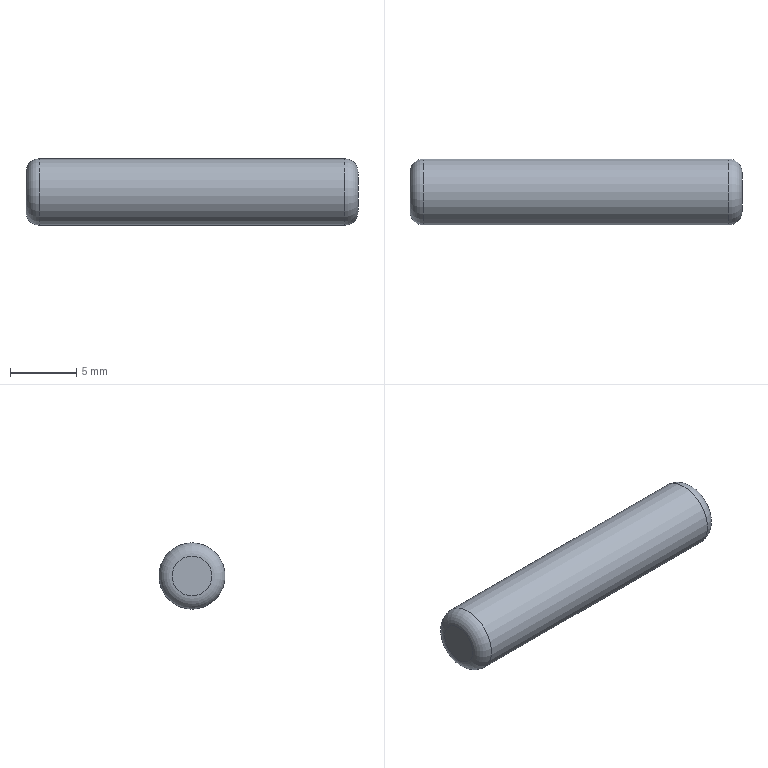Part | STEP file | 1 solid | 5 faces | box 25 x 5 x 5 mm | volume 484.734 mm3 | plane 2 | torus 2 | cylinder 1 | commonest cylinder face diameters 5 x1
STEP:
#1=CARTESIAN_POINT('',(0.,0.,0.));
#2=DIRECTION('',(0.,0.,1.));
#3=DIRECTION('',(1.,0.,0.));
#4=AXIS2_PLACEMENT_3D('',#1,#2,#3);
#5=CARTESIAN_POINT('',(1829.907,512.48,16.814));
#6=VERTEX_POINT('',#5);
#7=CARTESIAN_POINT('',(1829.907,512.48,15.314));
#8=DIRECTION('',(1.,0.,0.));
#9=DIRECTION('',(0.,0.,1.));
#10=AXIS2_PLACEMENT_3D('',#7,#8,#9);
#11=CIRCLE('',#10,1.5);
#12=CARTESIAN_POINT('',(1829.907,512.48,15.314));
#13=DIRECTION('',(1.,0.,0.));
#14=DIRECTION('',(0.,0.,-1.));
#15=AXIS2_PLACEMENT_3D('',#12,#13,#14);
#16=PLANE('',#15);
#17=CARTESIAN_POINT('',(0.,0.));
#18=DIRECTION('',(-1.,0.));
#19=AXIS2_PLACEMENT_2D('',#17,#18);
#20=CIRCLE('',#19,1.5);
#21=(GEOMETRIC_REPRESENTATION_CONTEXT(2)PARAMETRIC_REPRESENTATION_CONTEXT()REPRESENTATION_CONTEXT('',''));
#22=DEFINITIONAL_REPRESENTATION('',(#20),#21);
#23=PCURVE('',#16,#22);
#24=CARTESIAN_POINT('',(1828.907,512.48,15.314));
#25=DIRECTION('',(1.,0.,0.));
#26=DIRECTION('',(0.,0.,-1.));
#27=AXIS2_PLACEMENT_3D('',#24,#25,#26);
#28=TOROIDAL_SURFACE('',#27,1.5,1.);
#29=CARTESIAN_POINT('',(3.142,7.854));
#30=DIRECTION('',(1.,0.));
#31=VECTOR('',#30,1.);
#32=LINE('',#29,#31);
#33=(GEOMETRIC_REPRESENTATION_CONTEXT(2)PARAMETRIC_REPRESENTATION_CONTEXT()REPRESENTATION_CONTEXT('',''));
#34=DEFINITIONAL_REPRESENTATION('',(#32),#33);
#35=PCURVE('',#28,#34);
#36=SURFACE_CURVE('',#11,(#23,#35),.PCURVE_S1.);
#37=EDGE_CURVE('',#6,#6,#36,.T.);
#38=ORIENTED_EDGE('',*,*,#37,.T.);
#39=EDGE_LOOP('',(#38));
#40=FACE_BOUND('',#39,.T.);
#41=ADVANCED_FACE('',(#40),#16,.T.);
#42=CARTESIAN_POINT('',(1804.907,512.48,13.814));
#43=VERTEX_POINT('',#42);
#44=CARTESIAN_POINT('',(1804.907,512.48,15.314));
#45=DIRECTION('',(-1.,0.,0.));
#46=DIRECTION('',(0.,0.,-1.));
#47=AXIS2_PLACEMENT_3D('',#44,#45,#46);
#48=CIRCLE('',#47,1.5);
#49=CARTESIAN_POINT('',(1804.907,512.48,15.314));
#50=DIRECTION('',(-1.,0.,0.));
#51=DIRECTION('',(0.,0.,1.));
#52=AXIS2_PLACEMENT_3D('',#49,#50,#51);
#53=PLANE('',#52);
#54=CARTESIAN_POINT('',(0.,0.));
#55=DIRECTION('',(-1.,0.));
#56=AXIS2_PLACEMENT_2D('',#54,#55);
#57=CIRCLE('',#56,1.5);
#58=(GEOMETRIC_REPRESENTATION_CONTEXT(2)PARAMETRIC_REPRESENTATION_CONTEXT()REPRESENTATION_CONTEXT('',''));
#59=DEFINITIONAL_REPRESENTATION('',(#57),#58);
#60=PCURVE('',#53,#59);
#61=CARTESIAN_POINT('',(1805.907,512.48,15.314));
#62=DIRECTION('',(-1.,0.,0.));
#63=DIRECTION('',(0.,0.,1.));
#64=AXIS2_PLACEMENT_3D('',#61,#62,#63);
#65=TOROIDAL_SURFACE('',#64,1.5,1.);
#66=CARTESIAN_POINT('',(3.142,7.854));
#67=DIRECTION('',(1.,0.));
#68=VECTOR('',#67,1.);
#69=LINE('',#66,#68);
#70=(GEOMETRIC_REPRESENTATION_CONTEXT(2)PARAMETRIC_REPRESENTATION_CONTEXT()REPRESENTATION_CONTEXT('',''));
#71=DEFINITIONAL_REPRESENTATION('',(#69),#70);
#72=PCURVE('',#65,#71);
#73=SURFACE_CURVE('',#48,(#60,#72),.PCURVE_S1.);
#74=EDGE_CURVE('',#43,#43,#73,.T.);
#75=ORIENTED_EDGE('',*,*,#74,.T.);
#76=EDGE_LOOP('',(#75));
#77=FACE_BOUND('',#76,.T.);
#78=ADVANCED_FACE('',(#77),#53,.T.);
#79=CARTESIAN_POINT('',(1828.907,512.48,17.814));
#80=VERTEX_POINT('',#79);
#81=CARTESIAN_POINT('',(1828.907,512.48,12.814));
#82=VERTEX_POINT('',#81);
#83=CARTESIAN_POINT('',(1828.907,512.48,15.314));
#84=DIRECTION('',(-1.,0.,0.));
#85=DIRECTION('',(0.,0.,1.));
#86=AXIS2_PLACEMENT_3D('',#83,#84,#85);
#87=CIRCLE('',#86,2.5);
#88=CARTESIAN_POINT('',(1824.907,512.48,15.314));
#89=DIRECTION('',(1.,0.,0.));
#90=DIRECTION('',(0.,0.,-1.));
#91=AXIS2_PLACEMENT_3D('',#88,#89,#90);
#92=CYLINDRICAL_SURFACE('',#91,2.5);
#93=CARTESIAN_POINT('',(3.142,4.));
#94=DIRECTION('',(-1.,0.));
#95=VECTOR('',#94,1.);
#96=LINE('',#93,#95);
#97=(GEOMETRIC_REPRESENTATION_CONTEXT(2)PARAMETRIC_REPRESENTATION_CONTEXT()REPRESENTATION_CONTEXT('',''));
#98=DEFINITIONAL_REPRESENTATION('',(#96),#97);
#99=PCURVE('',#92,#98);
#100=CARTESIAN_POINT('',(9.425,6.283));
#101=DIRECTION('',(-1.,0.));
#102=VECTOR('',#101,1.);
#103=LINE('',#100,#102);
#104=(GEOMETRIC_REPRESENTATION_CONTEXT(2)PARAMETRIC_REPRESENTATION_CONTEXT()REPRESENTATION_CONTEXT('',''));
#105=DEFINITIONAL_REPRESENTATION('',(#103),#104);
#106=PCURVE('',#28,#105);
#107=SURFACE_CURVE('',#87,(#99,#106),.PCURVE_S1.);
#108=EDGE_CURVE('',#80,#82,#107,.T.);
#109=ORIENTED_EDGE('',*,*,#108,.T.);
#110=CARTESIAN_POINT('',(1805.907,512.48,12.814));
#111=VERTEX_POINT('',#110);
#112=CARTESIAN_POINT('',(1805.907,512.48,12.814));
#113=CARTESIAN_POINT('',(1828.907,512.48,12.814));
#114=B_SPLINE_CURVE_WITH_KNOTS('',1,(#112,#113),.UNSPECIFIED.,.F.,.F.,(2,2),(-19.,4.),.PIECEWISE_BEZIER_KNOTS.);
#115=CARTESIAN_POINT('',(0.,0.));
#116=DIRECTION('',(0.,1.));
#117=VECTOR('',#116,1.);
#118=LINE('',#115,#117);
#119=(GEOMETRIC_REPRESENTATION_CONTEXT(2)PARAMETRIC_REPRESENTATION_CONTEXT()REPRESENTATION_CONTEXT('',''));
#120=DEFINITIONAL_REPRESENTATION('',(#118),#119);
#121=PCURVE('',#92,#120);
#122=CARTESIAN_POINT('',(6.283,0.));
#123=DIRECTION('',(0.,1.));
#124=VECTOR('',#123,1.);
#125=LINE('',#122,#124);
#126=(GEOMETRIC_REPRESENTATION_CONTEXT(2)PARAMETRIC_REPRESENTATION_CONTEXT()REPRESENTATION_CONTEXT('',''));
#127=DEFINITIONAL_REPRESENTATION('',(#125),#126);
#128=PCURVE('',#92,#127);
#129=SEAM_CURVE('',#114,(#121,#128),.PCURVE_S1.);
#130=EDGE_CURVE('',#111,#82,#129,.T.);
#131=ORIENTED_EDGE('',*,*,#130,.F.);
#132=CARTESIAN_POINT('',(1805.907,512.48,15.314));
#133=DIRECTION('',(1.,0.,0.));
#134=DIRECTION('',(0.,0.,-1.));
#135=AXIS2_PLACEMENT_3D('',#132,#133,#134);
#136=CIRCLE('',#135,2.5);
#137=CARTESIAN_POINT('',(0.,-19.));
#138=DIRECTION('',(1.,0.));
#139=VECTOR('',#138,1.);
#140=LINE('',#137,#139);
#141=(GEOMETRIC_REPRESENTATION_CONTEXT(2)PARAMETRIC_REPRESENTATION_CONTEXT()REPRESENTATION_CONTEXT('',''));
#142=DEFINITIONAL_REPRESENTATION('',(#140),#141);
#143=PCURVE('',#92,#142);
#144=CARTESIAN_POINT('',(9.425,6.283));
#145=DIRECTION('',(-1.,0.));
#146=VECTOR('',#145,1.);
#147=LINE('',#144,#146);
#148=(GEOMETRIC_REPRESENTATION_CONTEXT(2)PARAMETRIC_REPRESENTATION_CONTEXT()REPRESENTATION_CONTEXT('',''));
#149=DEFINITIONAL_REPRESENTATION('',(#147),#148);
#150=PCURVE('',#65,#149);
#151=SURFACE_CURVE('',#136,(#143,#150),.PCURVE_S1.);
#152=EDGE_CURVE('',#111,#111,#151,.T.);
#153=ORIENTED_EDGE('',*,*,#152,.T.);
#154=ORIENTED_EDGE('',*,*,#130,.T.);
#155=CARTESIAN_POINT('',(1828.907,512.48,15.314));
#156=DIRECTION('',(-1.,0.,0.));
#157=DIRECTION('',(0.,0.,1.));
#158=AXIS2_PLACEMENT_3D('',#155,#156,#157);
#159=CIRCLE('',#158,2.5);
#160=CARTESIAN_POINT('',(9.425,4.));
#161=DIRECTION('',(-1.,0.));
#162=VECTOR('',#161,1.);
#163=LINE('',#160,#162);
#164=(GEOMETRIC_REPRESENTATION_CONTEXT(2)PARAMETRIC_REPRESENTATION_CONTEXT()REPRESENTATION_CONTEXT('',''));
#165=DEFINITIONAL_REPRESENTATION('',(#163),#164);
#166=PCURVE('',#92,#165);
#167=CARTESIAN_POINT('',(9.425,6.283));
#168=DIRECTION('',(-1.,0.));
#169=VECTOR('',#168,1.);
#170=LINE('',#167,#169);
#171=(GEOMETRIC_REPRESENTATION_CONTEXT(2)PARAMETRIC_REPRESENTATION_CONTEXT()REPRESENTATION_CONTEXT('',''));
#172=DEFINITIONAL_REPRESENTATION('',(#170),#171);
#173=PCURVE('',#28,#172);
#174=SURFACE_CURVE('',#159,(#166,#173),.PCURVE_S1.);
#175=EDGE_CURVE('',#82,#80,#174,.T.);
#176=ORIENTED_EDGE('',*,*,#175,.T.);
#177=EDGE_LOOP('',(#109,#131,#153,#154,#176));
#178=FACE_BOUND('',#177,.T.);
#179=ADVANCED_FACE('',(#178),#92,.T.);
#180=ORIENTED_EDGE('',*,*,#37,.F.);
#181=CARTESIAN_POINT('',(1828.907,512.48,17.814));
#182=CARTESIAN_POINT('',(1829.175,512.48,17.814));
#183=CARTESIAN_POINT('',(1829.435,512.48,17.729));
#184=CARTESIAN_POINT('',(1829.659,512.48,17.566));
#185=CARTESIAN_POINT('',(1829.822,512.48,17.342));
#186=CARTESIAN_POINT('',(1829.907,512.48,17.081));
#187=CARTESIAN_POINT('',(1829.907,512.48,16.814));
#188=(BOUNDED_CURVE()B_SPLINE_CURVE(6,(#181,#182,#183,#184,#185,#186,#187),.UNSPECIFIED.,.F.,.F.)B_SPLINE_CURVE_WITH_KNOTS((7,7),(0.,1.571),.PIECEWISE_BEZIER_KNOTS.)CURVE()GEOMETRIC_REPRESENTATION_ITEM()RATIONAL_B_SPLINE_CURVE((1.031,1.01,0.9979,0.994,0.9979,1.01,1.031))REPRESENTATION_ITEM(''));
#189=CARTESIAN_POINT('',(3.142,6.283));
#190=DIRECTION('',(0.,1.));
#191=VECTOR('',#190,1.);
#192=LINE('',#189,#191);
#193=(GEOMETRIC_REPRESENTATION_CONTEXT(2)PARAMETRIC_REPRESENTATION_CONTEXT()REPRESENTATION_CONTEXT('',''));
#194=DEFINITIONAL_REPRESENTATION('',(#192),#193);
#195=PCURVE('',#28,#194);
#196=CARTESIAN_POINT('',(9.425,6.283));
#197=DIRECTION('',(0.,1.));
#198=VECTOR('',#197,1.);
#199=LINE('',#196,#198);
#200=(GEOMETRIC_REPRESENTATION_CONTEXT(2)PARAMETRIC_REPRESENTATION_CONTEXT()REPRESENTATION_CONTEXT('',''));
#201=DEFINITIONAL_REPRESENTATION('',(#199),#200);
#202=PCURVE('',#28,#201);
#203=SEAM_CURVE('',#188,(#195,#202),.PCURVE_S1.);
#204=EDGE_CURVE('',#80,#6,#203,.T.);
#205=ORIENTED_EDGE('',*,*,#204,.F.);
#206=ORIENTED_EDGE('',*,*,#175,.F.);
#207=ORIENTED_EDGE('',*,*,#108,.F.);
#208=ORIENTED_EDGE('',*,*,#204,.T.);
#209=EDGE_LOOP('',(#180,#205,#206,#207,#208));
#210=FACE_BOUND('',#209,.T.);
#211=ADVANCED_FACE('',(#210),#28,.T.);
#212=ORIENTED_EDGE('',*,*,#74,.F.);
#213=CARTESIAN_POINT('',(1805.907,512.48,12.814));
#214=CARTESIAN_POINT('',(1805.64,512.48,12.814));
#215=CARTESIAN_POINT('',(1805.379,512.48,12.899));
#216=CARTESIAN_POINT('',(1805.155,512.48,13.062));
#217=CARTESIAN_POINT('',(1804.992,512.48,13.286));
#218=CARTESIAN_POINT('',(1804.907,512.48,13.547));
#219=CARTESIAN_POINT('',(1804.907,512.48,13.814));
#220=(BOUNDED_CURVE()B_SPLINE_CURVE(6,(#213,#214,#215,#216,#217,#218,#219),.UNSPECIFIED.,.F.,.F.)B_SPLINE_CURVE_WITH_KNOTS((7,7),(0.,1.571),.PIECEWISE_BEZIER_KNOTS.)CURVE()GEOMETRIC_REPRESENTATION_ITEM()RATIONAL_B_SPLINE_CURVE((1.031,1.01,0.9979,0.994,0.9979,1.01,1.031))REPRESENTATION_ITEM(''));
#221=CARTESIAN_POINT('',(3.142,6.283));
#222=DIRECTION('',(0.,1.));
#223=VECTOR('',#222,1.);
#224=LINE('',#221,#223);
#225=(GEOMETRIC_REPRESENTATION_CONTEXT(2)PARAMETRIC_REPRESENTATION_CONTEXT()REPRESENTATION_CONTEXT('',''));
#226=DEFINITIONAL_REPRESENTATION('',(#224),#225);
#227=PCURVE('',#65,#226);
#228=CARTESIAN_POINT('',(9.425,6.283));
#229=DIRECTION('',(0.,1.));
#230=VECTOR('',#229,1.);
#231=LINE('',#228,#230);
#232=(GEOMETRIC_REPRESENTATION_CONTEXT(2)PARAMETRIC_REPRESENTATION_CONTEXT()REPRESENTATION_CONTEXT('',''));
#233=DEFINITIONAL_REPRESENTATION('',(#231),#232);
#234=PCURVE('',#65,#233);
#235=SEAM_CURVE('',#220,(#227,#234),.PCURVE_S1.);
#236=EDGE_CURVE('',#111,#43,#235,.T.);
#237=ORIENTED_EDGE('',*,*,#236,.F.);
#238=ORIENTED_EDGE('',*,*,#152,.F.);
#239=ORIENTED_EDGE('',*,*,#236,.T.);
#240=EDGE_LOOP('',(#212,#237,#238,#239));
#241=FACE_BOUND('',#240,.T.);
#242=ADVANCED_FACE('',(#241),#65,.T.);
#243=CLOSED_SHELL('',(#41,#78,#179,#211,#242));
#244=MANIFOLD_SOLID_BREP('',#243);
#245=(LENGTH_UNIT()NAMED_UNIT(*)SI_UNIT(.MILLI.,.METRE.));
#246=UNCERTAINTY_MEASURE_WITH_UNIT(LENGTH_MEASURE(0.00001),#245,'','');
#247=(NAMED_UNIT(*)PLANE_ANGLE_UNIT()SI_UNIT($,.RADIAN.));
#248=(NAMED_UNIT(*)SI_UNIT($,.STERADIAN.)SOLID_ANGLE_UNIT());
#249=(GEOMETRIC_REPRESENTATION_CONTEXT(3)GLOBAL_UNCERTAINTY_ASSIGNED_CONTEXT((#246))GLOBAL_UNIT_ASSIGNED_CONTEXT((#245,#247,#248))REPRESENTATION_CONTEXT('',''));
#250=ADVANCED_BREP_SHAPE_REPRESENTATION('',(#4,#244),#249);